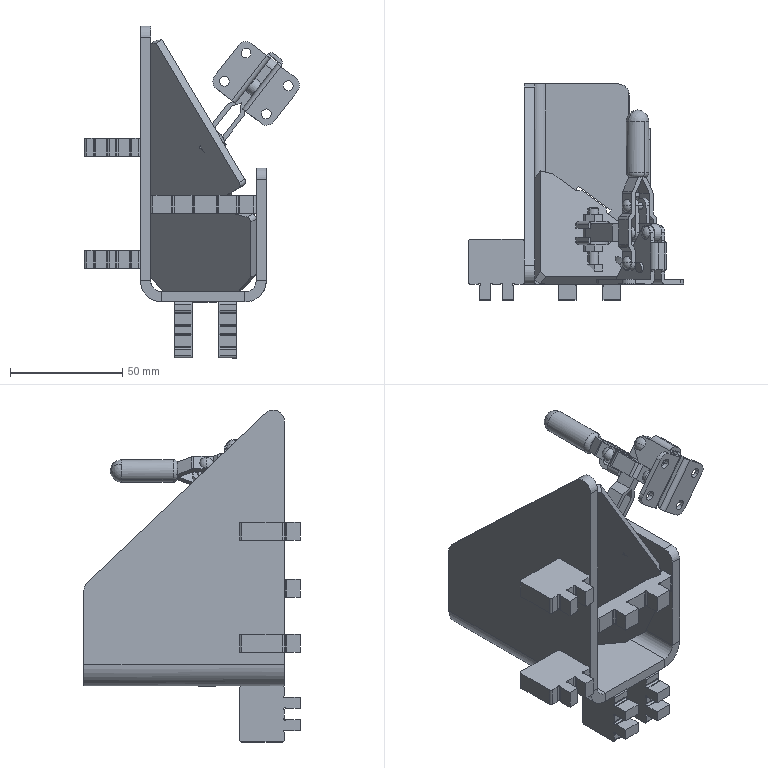Part | SolidWorks | features LocalLPattern 2, ReferencePattern 2 | 12 solids | 514 faces | box 95.955 x 96.4 x 148.047 mm | volume 120880 mm3 | plane 246 | cylinder 207 | cone 41 | sphere 18 | torus 2 | commonest cylinder face diameters 2 x66 1 x34 3 x26 4 x11 10 x11 7 x10